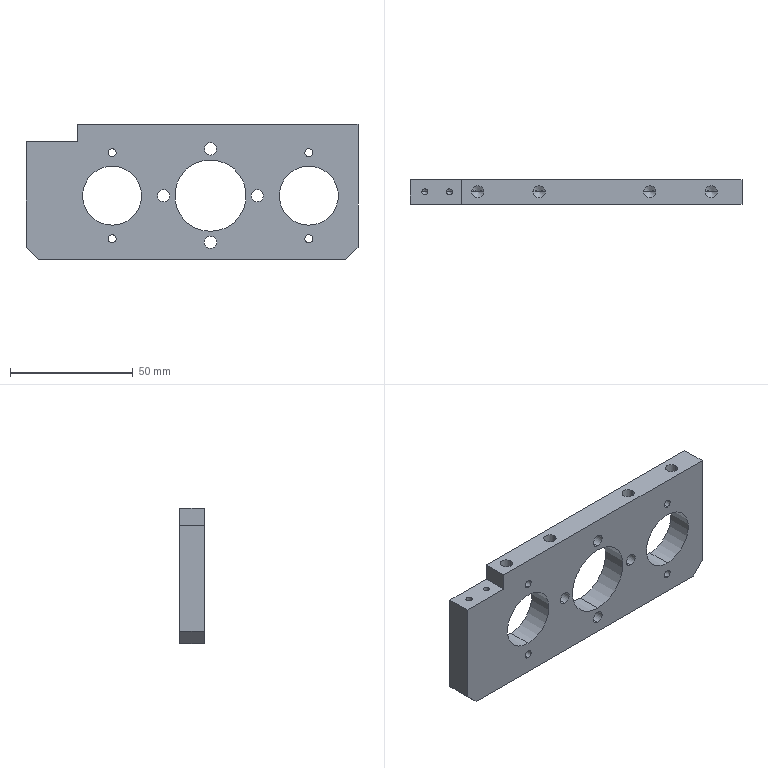Part | STEP file | 0232_205_Plate | 1 solid | 56 faces | box 135 x 10 x 55 mm | volume 54422 mm3 | cylinder 34 | cone 12 | plane 10 | commonest cylinder face diameters 5 x16 3.3 x8 2.5 x4 24 x4 29 x2